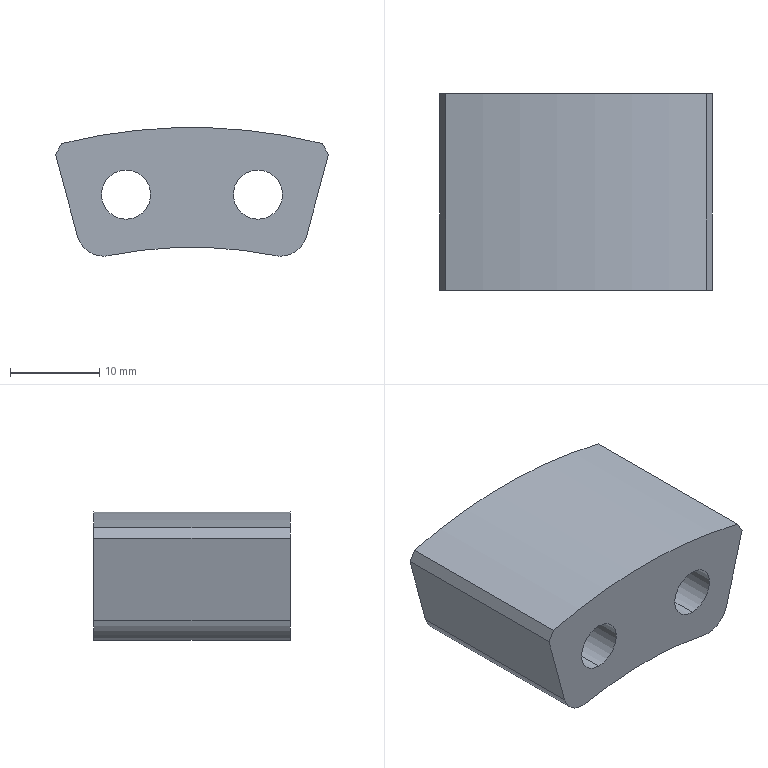Part | SolidWorks | features Chamfer 1, Extrusion 1, Fillet 1, HoleWzd 1, ICE 1 | 1 solid | 22 faces | box 30.541 x 22 x 14.401 mm | volume 6316 mm3 | cylinder 14 | plane 8 | commonest cylinder face diameters 5.5 x4 6 x4 10 x4 93.2 x1 120 x1
STEP:
#1=CARTESIAN_POINT('',(-7.376,15.,47.484));
#2=VERTEX_POINT('',#1);
#3=CARTESIAN_POINT('',(-7.376,15.,57.484));
#4=VERTEX_POINT('',#3);
#5=CARTESIAN_POINT('',(-7.376,15.,52.484));
#6=DIRECTION('',(0.,1.,0.));
#7=DIRECTION('',(0.,0.,1.));
#8=AXIS2_PLACEMENT_3D('',#5,#6,#7);
#9=CIRCLE('',#8,5.);
#10=EDGE_CURVE('',#2,#4,#9,.T.);
#11=ORIENTED_EDGE('',*,*,#10,.F.);
#12=CARTESIAN_POINT('',(-7.376,22.,47.484));
#13=VERTEX_POINT('',#12);
#14=CARTESIAN_POINT('',(-7.376,22.,47.484));
#15=DIRECTION('',(0.,1.,0.));
#16=VECTOR('',#15,1000.);
#17=LINE('',#14,#16);
#18=EDGE_CURVE('',#2,#13,#17,.T.);
#19=ORIENTED_EDGE('',*,*,#18,.T.);
#20=CARTESIAN_POINT('',(-7.376,22.,57.484));
#21=VERTEX_POINT('',#20);
#22=CARTESIAN_POINT('',(-7.376,22.,52.484));
#23=DIRECTION('',(0.,1.,0.));
#24=DIRECTION('',(0.,0.,1.));
#25=AXIS2_PLACEMENT_3D('',#22,#23,#24);
#26=CIRCLE('',#25,5.);
#27=EDGE_CURVE('',#13,#21,#26,.T.);
#28=ORIENTED_EDGE('',*,*,#27,.T.);
#29=CARTESIAN_POINT('',(-7.376,22.,57.484));
#30=DIRECTION('',(0.,1.,0.));
#31=VECTOR('',#30,1000.);
#32=LINE('',#29,#31);
#33=EDGE_CURVE('',#4,#21,#32,.T.);
#34=ORIENTED_EDGE('',*,*,#33,.F.);
#35=EDGE_LOOP('',(#11,#19,#28,#34));
#36=FACE_OUTER_BOUND('',#35,.T.);
#37=CARTESIAN_POINT('',(-7.376,22.,52.484));
#38=DIRECTION('',(0.,1.,0.));
#39=DIRECTION('',(0.,0.,1.));
#40=AXIS2_PLACEMENT_3D('',#37,#38,#39);
#41=CYLINDRICAL_SURFACE('',#40,5.);
#42=ADVANCED_FACE('',(#36),#41,.F.);
#43=CARTESIAN_POINT('',(-7.376,0.,49.734));
#44=VERTEX_POINT('',#43);
#45=CARTESIAN_POINT('',(-7.376,0.,55.234));
#46=VERTEX_POINT('',#45);
#47=CARTESIAN_POINT('',(-7.376,0.,52.484));
#48=DIRECTION('',(0.,1.,0.));
#49=DIRECTION('',(0.,0.,1.));
#50=AXIS2_PLACEMENT_3D('',#47,#48,#49);
#51=CIRCLE('',#50,2.75);
#52=EDGE_CURVE('',#44,#46,#51,.T.);
#53=ORIENTED_EDGE('',*,*,#52,.F.);
#54=CARTESIAN_POINT('',(-7.376,15.,49.734));
#55=VERTEX_POINT('',#54);
#56=CARTESIAN_POINT('',(-7.376,22.,49.734));
#57=DIRECTION('',(0.,1.,0.));
#58=VECTOR('',#57,1000.);
#59=LINE('',#56,#58);
#60=EDGE_CURVE('',#44,#55,#59,.T.);
#61=ORIENTED_EDGE('',*,*,#60,.T.);
#62=CARTESIAN_POINT('',(-7.376,15.,55.234));
#63=VERTEX_POINT('',#62);
#64=CARTESIAN_POINT('',(-7.376,15.,52.484));
#65=DIRECTION('',(0.,1.,0.));
#66=DIRECTION('',(0.,0.,1.));
#67=AXIS2_PLACEMENT_3D('',#64,#65,#66);
#68=CIRCLE('',#67,2.75);
#69=EDGE_CURVE('',#55,#63,#68,.T.);
#70=ORIENTED_EDGE('',*,*,#69,.T.);
#71=CARTESIAN_POINT('',(-7.376,22.,55.234));
#72=DIRECTION('',(0.,1.,0.));
#73=VECTOR('',#72,1000.);
#74=LINE('',#71,#73);
#75=EDGE_CURVE('',#46,#63,#74,.T.);
#76=ORIENTED_EDGE('',*,*,#75,.F.);
#77=EDGE_LOOP('',(#53,#61,#70,#76));
#78=FACE_OUTER_BOUND('',#77,.T.);
#79=CARTESIAN_POINT('',(-7.376,22.,52.484));
#80=DIRECTION('',(0.,1.,0.));
#81=DIRECTION('',(0.,0.,1.));
#82=AXIS2_PLACEMENT_3D('',#79,#80,#81);
#83=CYLINDRICAL_SURFACE('',#82,2.75);
#84=ADVANCED_FACE('',(#78),#83,.F.);
#85=CARTESIAN_POINT('',(7.376,15.,47.484));
#86=VERTEX_POINT('',#85);
#87=CARTESIAN_POINT('',(7.376,15.,57.484));
#88=VERTEX_POINT('',#87);
#89=CARTESIAN_POINT('',(7.376,15.,52.484));
#90=DIRECTION('',(0.,1.,0.));
#91=DIRECTION('',(0.,0.,1.));
#92=AXIS2_PLACEMENT_3D('',#89,#90,#91);
#93=CIRCLE('',#92,5.);
#94=EDGE_CURVE('',#86,#88,#93,.T.);
#95=ORIENTED_EDGE('',*,*,#94,.F.);
#96=CARTESIAN_POINT('',(7.376,22.,47.484));
#97=VERTEX_POINT('',#96);
#98=CARTESIAN_POINT('',(7.376,22.,47.484));
#99=DIRECTION('',(0.,1.,0.));
#100=VECTOR('',#99,1000.);
#101=LINE('',#98,#100);
#102=EDGE_CURVE('',#86,#97,#101,.T.);
#103=ORIENTED_EDGE('',*,*,#102,.T.);
#104=CARTESIAN_POINT('',(7.376,22.,57.484));
#105=VERTEX_POINT('',#104);
#106=CARTESIAN_POINT('',(7.376,22.,52.484));
#107=DIRECTION('',(0.,1.,0.));
#108=DIRECTION('',(0.,0.,1.));
#109=AXIS2_PLACEMENT_3D('',#106,#107,#108);
#110=CIRCLE('',#109,5.);
#111=EDGE_CURVE('',#97,#105,#110,.T.);
#112=ORIENTED_EDGE('',*,*,#111,.T.);
#113=CARTESIAN_POINT('',(7.376,22.,57.484));
#114=DIRECTION('',(0.,1.,0.));
#115=VECTOR('',#114,1000.);
#116=LINE('',#113,#115);
#117=EDGE_CURVE('',#88,#105,#116,.T.);
#118=ORIENTED_EDGE('',*,*,#117,.F.);
#119=EDGE_LOOP('',(#95,#103,#112,#118));
#120=FACE_OUTER_BOUND('',#119,.T.);
#121=CARTESIAN_POINT('',(7.376,22.,52.484));
#122=DIRECTION('',(0.,1.,0.));
#123=DIRECTION('',(0.,0.,1.));
#124=AXIS2_PLACEMENT_3D('',#121,#122,#123);
#125=CYLINDRICAL_SURFACE('',#124,5.);
#126=ADVANCED_FACE('',(#120),#125,.F.);
#127=CARTESIAN_POINT('',(7.376,0.,49.734));
#128=VERTEX_POINT('',#127);
#129=CARTESIAN_POINT('',(7.376,0.,55.234));
#130=VERTEX_POINT('',#129);
#131=CARTESIAN_POINT('',(7.376,0.,52.484));
#132=DIRECTION('',(0.,1.,0.));
#133=DIRECTION('',(0.,0.,1.));
#134=AXIS2_PLACEMENT_3D('',#131,#132,#133);
#135=CIRCLE('',#134,2.75);
#136=EDGE_CURVE('',#128,#130,#135,.T.);
#137=ORIENTED_EDGE('',*,*,#136,.F.);
#138=CARTESIAN_POINT('',(7.376,15.,49.734));
#139=VERTEX_POINT('',#138);
#140=CARTESIAN_POINT('',(7.376,22.,49.734));
#141=DIRECTION('',(0.,1.,0.));
#142=VECTOR('',#141,1000.);
#143=LINE('',#140,#142);
#144=EDGE_CURVE('',#128,#139,#143,.T.);
#145=ORIENTED_EDGE('',*,*,#144,.T.);
#146=CARTESIAN_POINT('',(7.376,15.,55.234));
#147=VERTEX_POINT('',#146);
#148=CARTESIAN_POINT('',(7.376,15.,52.484));
#149=DIRECTION('',(0.,1.,0.));
#150=DIRECTION('',(0.,0.,1.));
#151=AXIS2_PLACEMENT_3D('',#148,#149,#150);
#152=CIRCLE('',#151,2.75);
#153=EDGE_CURVE('',#139,#147,#152,.T.);
#154=ORIENTED_EDGE('',*,*,#153,.T.);
#155=CARTESIAN_POINT('',(7.376,22.,55.234));
#156=DIRECTION('',(0.,1.,0.));
#157=VECTOR('',#156,1000.);
#158=LINE('',#155,#157);
#159=EDGE_CURVE('',#130,#147,#158,.T.);
#160=ORIENTED_EDGE('',*,*,#159,.F.);
#161=EDGE_LOOP('',(#137,#145,#154,#160));
#162=FACE_OUTER_BOUND('',#161,.T.);
#163=CARTESIAN_POINT('',(7.376,22.,52.484));
#164=DIRECTION('',(0.,1.,0.));
#165=DIRECTION('',(0.,0.,1.));
#166=AXIS2_PLACEMENT_3D('',#163,#164,#165);
#167=CYLINDRICAL_SURFACE('',#166,2.75);
#168=ADVANCED_FACE('',(#162),#167,.F.);
#169=CARTESIAN_POINT('',(9.916,22.,45.599));
#170=VERTEX_POINT('',#169);
#171=CARTESIAN_POINT('',(9.316,22.,45.659));
#172=VERTEX_POINT('',#171);
#173=CARTESIAN_POINT('',(9.916,22.,48.599));
#174=DIRECTION('',(0.,1.,0.));
#175=DIRECTION('',(0.,0.,1.));
#176=AXIS2_PLACEMENT_3D('',#173,#174,#175);
#177=CIRCLE('',#176,3.);
#178=EDGE_CURVE('',#170,#172,#177,.T.);
#179=ORIENTED_EDGE('',*,*,#178,.F.);
#180=CARTESIAN_POINT('',(9.916,0.,45.599));
#181=VERTEX_POINT('',#180);
#182=CARTESIAN_POINT('',(9.916,22.,45.599));
#183=DIRECTION('',(0.,-1.,0.));
#184=VECTOR('',#183,1000.);
#185=LINE('',#182,#184);
#186=EDGE_CURVE('',#170,#181,#185,.T.);
#187=ORIENTED_EDGE('',*,*,#186,.T.);
#188=CARTESIAN_POINT('',(9.316,0.,45.659));
#189=VERTEX_POINT('',#188);
#190=CARTESIAN_POINT('',(9.916,0.,48.599));
#191=DIRECTION('',(0.,-1.,0.));
#192=DIRECTION('',(0.,0.,1.));
#193=AXIS2_PLACEMENT_3D('',#190,#191,#192);
#194=CIRCLE('',#193,3.);
#195=EDGE_CURVE('',#189,#181,#194,.T.);
#196=ORIENTED_EDGE('',*,*,#195,.F.);
#197=CARTESIAN_POINT('',(9.316,22.,45.659));
#198=DIRECTION('',(0.,-1.,0.));
#199=VECTOR('',#198,1000.);
#200=LINE('',#197,#199);
#201=EDGE_CURVE('',#172,#189,#200,.T.);
#202=ORIENTED_EDGE('',*,*,#201,.F.);
#203=EDGE_LOOP('',(#179,#187,#196,#202));
#204=FACE_OUTER_BOUND('',#203,.T.);
#205=CARTESIAN_POINT('',(9.916,22.,48.599));
#206=DIRECTION('',(0.,-1.,0.));
#207=DIRECTION('',(0.,0.,-1.));
#208=AXIS2_PLACEMENT_3D('',#205,#206,#207);
#209=CYLINDRICAL_SURFACE('',#208,3.);
#210=ADVANCED_FACE('',(#204),#209,.T.);
#211=CARTESIAN_POINT('',(-9.916,22.,45.599));
#212=VERTEX_POINT('',#211);
#213=CARTESIAN_POINT('',(-12.814,22.,47.822));
#214=VERTEX_POINT('',#213);
#215=CARTESIAN_POINT('',(-9.916,22.,48.599));
#216=DIRECTION('',(0.,1.,0.));
#217=DIRECTION('',(0.,0.,1.));
#218=AXIS2_PLACEMENT_3D('',#215,#216,#217);
#219=CIRCLE('',#218,3.);
#220=EDGE_CURVE('',#212,#214,#219,.T.);
#221=ORIENTED_EDGE('',*,*,#220,.F.);
#222=CARTESIAN_POINT('',(-9.916,0.,45.599));
#223=VERTEX_POINT('',#222);
#224=CARTESIAN_POINT('',(-9.916,22.,45.599));
#225=DIRECTION('',(0.,-1.,0.));
#226=VECTOR('',#225,1000.);
#227=LINE('',#224,#226);
#228=EDGE_CURVE('',#212,#223,#227,.T.);
#229=ORIENTED_EDGE('',*,*,#228,.T.);
#230=CARTESIAN_POINT('',(-12.814,0.,47.822));
#231=VERTEX_POINT('',#230);
#232=CARTESIAN_POINT('',(-9.916,0.,48.599));
#233=DIRECTION('',(0.,-1.,0.));
#234=DIRECTION('',(0.,0.,1.));
#235=AXIS2_PLACEMENT_3D('',#232,#233,#234);
#236=CIRCLE('',#235,3.);
#237=EDGE_CURVE('',#231,#223,#236,.T.);
#238=ORIENTED_EDGE('',*,*,#237,.F.);
#239=CARTESIAN_POINT('',(-12.814,0.,47.822));
#240=DIRECTION('',(0.,-1.,0.));
#241=VECTOR('',#240,1000.);
#242=LINE('',#239,#241);
#243=EDGE_CURVE('',#214,#231,#242,.T.);
#244=ORIENTED_EDGE('',*,*,#243,.F.);
#245=EDGE_LOOP('',(#221,#229,#238,#244));
#246=FACE_OUTER_BOUND('',#245,.T.);
#247=CARTESIAN_POINT('',(-9.916,22.,48.599));
#248=DIRECTION('',(0.,-1.,0.));
#249=DIRECTION('',(0.,0.,-1.));
#250=AXIS2_PLACEMENT_3D('',#247,#248,#249);
#251=CYLINDRICAL_SURFACE('',#250,3.);
#252=ADVANCED_FACE('',(#246),#251,.T.);
#253=CARTESIAN_POINT('',(-7.376,22.,52.484));
#254=DIRECTION('',(0.,1.,0.));
#255=DIRECTION('',(0.,0.,1.));
#256=AXIS2_PLACEMENT_3D('',#253,#254,#255);
#257=CIRCLE('',#256,5.);
#258=EDGE_CURVE('',#21,#13,#257,.T.);
#259=ORIENTED_EDGE('',*,*,#258,.F.);
#260=ORIENTED_EDGE('',*,*,#27,.F.);
#261=EDGE_LOOP('',(#259,#260));
#262=FACE_BOUND('',#261,.T.);
#263=CARTESIAN_POINT('',(7.376,22.,52.484));
#264=DIRECTION('',(0.,1.,0.));
#265=DIRECTION('',(0.,0.,1.));
#266=AXIS2_PLACEMENT_3D('',#263,#264,#265);
#267=CIRCLE('',#266,5.);
#268=EDGE_CURVE('',#105,#97,#267,.T.);
#269=ORIENTED_EDGE('',*,*,#268,.F.);
#270=ORIENTED_EDGE('',*,*,#111,.F.);
#271=EDGE_LOOP('',(#269,#270));
#272=FACE_BOUND('',#271,.T.);
#273=CARTESIAN_POINT('',(-15.27,22.,56.99));
#274=VERTEX_POINT('',#273);
#275=CARTESIAN_POINT('',(-12.061,22.,45.012));
#276=DIRECTION('',(-0.2588,0.,0.9659));
#277=VECTOR('',#276,1000.);
#278=LINE('',#275,#277);
#279=EDGE_CURVE('',#214,#274,#278,.T.);
#280=ORIENTED_EDGE('',*,*,#279,.T.);
#281=CARTESIAN_POINT('',(-14.569,22.,58.204));
#282=VERTEX_POINT('',#281);
#283=CARTESIAN_POINT('',(-36.13,22.,20.86));
#284=DIRECTION('',(0.5,0.,0.866));
#285=VECTOR('',#284,1000.);
#286=LINE('',#283,#285);
#287=EDGE_CURVE('',#274,#282,#286,.T.);
#288=ORIENTED_EDGE('',*,*,#287,.T.);
#289=CARTESIAN_POINT('',(14.569,22.,58.204));
#290=VERTEX_POINT('',#289);
#291=CARTESIAN_POINT('',(0.,22.,0.));
#292=DIRECTION('',(0.,1.,0.));
#293=DIRECTION('',(0.,0.,1.));
#294=AXIS2_PLACEMENT_3D('',#291,#292,#293);
#295=CIRCLE('',#294,60.);
#296=EDGE_CURVE('',#282,#290,#295,.T.);
#297=ORIENTED_EDGE('',*,*,#296,.T.);
#298=CARTESIAN_POINT('',(15.27,22.,56.99));
#299=VERTEX_POINT('',#298);
#300=CARTESIAN_POINT('',(36.13,22.,20.86));
#301=DIRECTION('',(0.5,0.,-0.866));
#302=VECTOR('',#301,1000.);
#303=LINE('',#300,#302);
#304=EDGE_CURVE('',#290,#299,#303,.T.);
#305=ORIENTED_EDGE('',*,*,#304,.T.);
#306=CARTESIAN_POINT('',(12.814,22.,47.822));
#307=VERTEX_POINT('',#306);
#308=CARTESIAN_POINT('',(12.061,22.,45.012));
#309=DIRECTION('',(-0.2588,0.,-0.9659));
#310=VECTOR('',#309,1000.);
#311=LINE('',#308,#310);
#312=EDGE_CURVE('',#299,#307,#311,.T.);
#313=ORIENTED_EDGE('',*,*,#312,.T.);
#314=CARTESIAN_POINT('',(9.916,22.,48.599));
#315=DIRECTION('',(0.,1.,0.));
#316=DIRECTION('',(0.,0.,1.));
#317=AXIS2_PLACEMENT_3D('',#314,#315,#316);
#318=CIRCLE('',#317,3.);
#319=EDGE_CURVE('',#307,#170,#318,.T.);
#320=ORIENTED_EDGE('',*,*,#319,.T.);
#321=ORIENTED_EDGE('',*,*,#178,.T.);
#322=CARTESIAN_POINT('',(-9.316,22.,45.659));
#323=VERTEX_POINT('',#322);
#324=CARTESIAN_POINT('',(0.,22.,0.));
#325=DIRECTION('',(0.,1.,0.));
#326=DIRECTION('',(0.,0.,1.));
#327=AXIS2_PLACEMENT_3D('',#324,#325,#326);
#328=CIRCLE('',#327,46.6);
#329=EDGE_CURVE('',#323,#172,#328,.T.);
#330=ORIENTED_EDGE('',*,*,#329,.F.);
#331=CARTESIAN_POINT('',(-9.916,22.,48.599));
#332=DIRECTION('',(0.,1.,0.));
#333=DIRECTION('',(0.,0.,1.));
#334=AXIS2_PLACEMENT_3D('',#331,#332,#333);
#335=CIRCLE('',#334,3.);
#336=EDGE_CURVE('',#323,#212,#335,.T.);
#337=ORIENTED_EDGE('',*,*,#336,.T.);
#338=ORIENTED_EDGE('',*,*,#220,.T.);
#339=EDGE_LOOP('',(#280,#288,#297,#305,#313,#320,#321,#330,#337,#338));
#340=FACE_OUTER_BOUND('',#339,.T.);
#341=CARTESIAN_POINT('',(0.,22.,0.));
#342=DIRECTION('',(0.,1.,0.));
#343=DIRECTION('',(0.,0.,1.));
#344=AXIS2_PLACEMENT_3D('',#341,#342,#343);
#345=PLANE('',#344);
#346=ADVANCED_FACE('',(#262,#272,#340),#345,.T.);
#347=CARTESIAN_POINT('',(-7.376,0.,52.484));
#348=DIRECTION('',(0.,1.,0.));
#349=DIRECTION('',(0.,0.,1.));
#350=AXIS2_PLACEMENT_3D('',#347,#348,#349);
#351=CIRCLE('',#350,2.75);
#352=EDGE_CURVE('',#46,#44,#351,.T.);
#353=ORIENTED_EDGE('',*,*,#352,.T.);
#354=ORIENTED_EDGE('',*,*,#52,.T.);
#355=EDGE_LOOP('',(#353,#354));
#356=FACE_BOUND('',#355,.T.);
#357=CARTESIAN_POINT('',(7.376,0.,52.484));
#358=DIRECTION('',(0.,1.,0.));
#359=DIRECTION('',(0.,0.,1.));
#360=AXIS2_PLACEMENT_3D('',#357,#358,#359);
#361=CIRCLE('',#360,2.75);
#362=EDGE_CURVE('',#130,#128,#361,.T.);
#363=ORIENTED_EDGE('',*,*,#362,.T.);
#364=ORIENTED_EDGE('',*,*,#136,.T.);
#365=EDGE_LOOP('',(#363,#364));
#366=FACE_BOUND('',#365,.T.);
#367=CARTESIAN_POINT('',(-14.569,0.,58.204));
#368=VERTEX_POINT('',#367);
#369=CARTESIAN_POINT('',(14.569,0.,58.204));
#370=VERTEX_POINT('',#369);
#371=CARTESIAN_POINT('',(0.,0.,0.));
#372=DIRECTION('',(0.,1.,0.));
#373=DIRECTION('',(0.,0.,1.));
#374=AXIS2_PLACEMENT_3D('',#371,#372,#373);
#375=CIRCLE('',#374,60.);
#376=EDGE_CURVE('',#368,#370,#375,.T.);
#377=ORIENTED_EDGE('',*,*,#376,.F.);
#378=CARTESIAN_POINT('',(-15.27,0.,56.99));
#379=VERTEX_POINT('',#378);
#380=CARTESIAN_POINT('',(-15.27,0.,56.99));
#381=DIRECTION('',(-0.5,0.,-0.866));
#382=VECTOR('',#381,1000.);
#383=LINE('',#380,#382);
#384=EDGE_CURVE('',#368,#379,#383,.T.);
#385=ORIENTED_EDGE('',*,*,#384,.T.);
#386=CARTESIAN_POINT('',(-12.061,0.,45.012));
#387=DIRECTION('',(-0.2588,0.,0.9659));
#388=VECTOR('',#387,1000.);
#389=LINE('',#386,#388);
#390=EDGE_CURVE('',#231,#379,#389,.T.);
#391=ORIENTED_EDGE('',*,*,#390,.F.);
#392=ORIENTED_EDGE('',*,*,#237,.T.);
#393=CARTESIAN_POINT('',(-9.316,0.,45.659));
#394=VERTEX_POINT('',#393);
#395=CARTESIAN_POINT('',(-9.916,0.,48.599));
#396=DIRECTION('',(0.,-1.,0.));
#397=DIRECTION('',(0.,0.,1.));
#398=AXIS2_PLACEMENT_3D('',#395,#396,#397);
#399=CIRCLE('',#398,3.);
#400=EDGE_CURVE('',#223,#394,#399,.T.);
#401=ORIENTED_EDGE('',*,*,#400,.T.);
#402=CARTESIAN_POINT('',(0.,0.,0.));
#403=DIRECTION('',(0.,1.,0.));
#404=DIRECTION('',(0.,0.,1.));
#405=AXIS2_PLACEMENT_3D('',#402,#403,#404);
#406=CIRCLE('',#405,46.6);
#407=EDGE_CURVE('',#394,#189,#406,.T.);
#408=ORIENTED_EDGE('',*,*,#407,.T.);
#409=ORIENTED_EDGE('',*,*,#195,.T.);
#410=CARTESIAN_POINT('',(12.814,0.,47.822));
#411=VERTEX_POINT('',#410);
#412=CARTESIAN_POINT('',(9.916,0.,48.599));
#413=DIRECTION('',(0.,-1.,0.));
#414=DIRECTION('',(0.,0.,1.));
#415=AXIS2_PLACEMENT_3D('',#412,#413,#414);
#416=CIRCLE('',#415,3.);
#417=EDGE_CURVE('',#181,#411,#416,.T.);
#418=ORIENTED_EDGE('',*,*,#417,.T.);
#419=CARTESIAN_POINT('',(15.27,0.,56.99));
#420=VERTEX_POINT('',#419);
#421=CARTESIAN_POINT('',(12.061,0.,45.012));
#422=DIRECTION('',(-0.2588,0.,-0.9659));
#423=VECTOR('',#422,1000.);
#424=LINE('',#421,#423);
#425=EDGE_CURVE('',#420,#411,#424,.T.);
#426=ORIENTED_EDGE('',*,*,#425,.F.);
#427=CARTESIAN_POINT('',(14.569,0.,58.204));
#428=DIRECTION('',(-0.5,0.,0.866));
#429=VECTOR('',#428,1000.);
#430=LINE('',#427,#429);
#431=EDGE_CURVE('',#420,#370,#430,.T.);
#432=ORIENTED_EDGE('',*,*,#431,.T.);
#433=EDGE_LOOP('',(#377,#385,#391,#392,#401,#408,#409,#418,#426,#432));
#434=FACE_OUTER_BOUND('',#433,.T.);
#435=CARTESIAN_POINT('',(0.,0.,0.));
#436=DIRECTION('',(0.,1.,0.));
#437=DIRECTION('',(0.,0.,1.));
#438=AXIS2_PLACEMENT_3D('',#435,#436,#437);
#439=PLANE('',#438);
#440=ADVANCED_FACE('',(#356,#366,#434),#439,.F.);
#441=ORIENTED_EDGE('',*,*,#296,.F.);
#442=CARTESIAN_POINT('',(-14.569,22.,58.204));
#443=DIRECTION('',(0.,-1.,0.));
#444=VECTOR('',#443,1000.);
#445=LINE('',#442,#444);
#446=EDGE_CURVE('',#282,#368,#445,.T.);
#447=ORIENTED_EDGE('',*,*,#446,.T.);
#448=ORIENTED_EDGE('',*,*,#376,.T.);
#449=CARTESIAN_POINT('',(14.569,22.,58.204));
#450=DIRECTION('',(0.,1.,0.));
#451=VECTOR('',#450,1000.);
#452=LINE('',#449,#451);
#453=EDGE_CURVE('',#370,#290,#452,.T.);
#454=ORIENTED_EDGE('',*,*,#453,.T.);
#455=EDGE_LOOP('',(#441,#447,#448,#454));
#456=FACE_OUTER_BOUND('',#455,.T.);
#457=CARTESIAN_POINT('',(0.,22.,0.));
#458=DIRECTION('',(0.,-1.,0.));
#459=DIRECTION('',(0.,0.,-1.));
#460=AXIS2_PLACEMENT_3D('',#457,#458,#459);
#461=CYLINDRICAL_SURFACE('',#460,60.);
#462=ADVANCED_FACE('',(#456),#461,.T.);
#463=ORIENTED_EDGE('',*,*,#407,.F.);
#464=CARTESIAN_POINT('',(-9.316,22.,45.659));
#465=DIRECTION('',(0.,1.,0.));
#466=VECTOR('',#465,1000.);
#467=LINE('',#464,#466);
#468=EDGE_CURVE('',#394,#323,#467,.T.);
#469=ORIENTED_EDGE('',*,*,#468,.T.);
#470=ORIENTED_EDGE('',*,*,#329,.T.);
#471=ORIENTED_EDGE('',*,*,#201,.T.);
#472=EDGE_LOOP('',(#463,#469,#470,#471));
#473=FACE_OUTER_BOUND('',#472,.T.);
#474=CARTESIAN_POINT('',(0.,22.,0.));
#475=DIRECTION('',(0.,-1.,0.));
#476=DIRECTION('',(0.,0.,-1.));
#477=AXIS2_PLACEMENT_3D('',#474,#475,#476);
#478=CYLINDRICAL_SURFACE('',#477,46.6);
#479=ADVANCED_FACE('',(#473),#478,.F.);
#480=ORIENTED_EDGE('',*,*,#312,.F.);
#481=CARTESIAN_POINT('',(15.27,0.,56.99));
#482=DIRECTION('',(0.,-1.,0.));
#483=VECTOR('',#482,1000.);
#484=LINE('',#481,#483);
#485=EDGE_CURVE('',#299,#420,#484,.T.);
#486=ORIENTED_EDGE('',*,*,#485,.T.);
#487=ORIENTED_EDGE('',*,*,#425,.T.);
#488=CARTESIAN_POINT('',(12.814,0.,47.822));
#489=DIRECTION('',(0.,1.,0.));
#490=VECTOR('',#489,1000.);
#491=LINE('',#488,#490);
#492=EDGE_CURVE('',#411,#307,#491,.T.);
#493=ORIENTED_EDGE('',*,*,#492,.T.);
#494=EDGE_LOOP('',(#480,#486,#487,#493));
#495=FACE_OUTER_BOUND('',#494,.T.);
#496=CARTESIAN_POINT('',(12.061,0.,45.012));
#497=DIRECTION('',(0.9659,0.,-0.2588));
#498=DIRECTION('',(-0.2588,0.,-0.9659));
#499=AXIS2_PLACEMENT_3D('',#496,#497,#498);
#500=PLANE('',#499);
#501=ADVANCED_FACE('',(#495),#500,.T.);
#502=ORIENTED_EDGE('',*,*,#390,.T.);
#503=CARTESIAN_POINT('',(-15.27,22.,56.99));
#504=DIRECTION('',(0.,1.,0.));
#505=VECTOR('',#504,1000.);
#506=LINE('',#503,#505);
#507=EDGE_CURVE('',#379,#274,#506,.T.);
#508=ORIENTED_EDGE('',*,*,#507,.T.);
#509=ORIENTED_EDGE('',*,*,#279,.F.);
#510=ORIENTED_EDGE('',*,*,#243,.T.);
#511=EDGE_LOOP('',(#502,#508,#509,#510));
#512=FACE_OUTER_BOUND('',#511,.T.);
#513=CARTESIAN_POINT('',(-12.061,0.,45.012));
#514=DIRECTION('',(-0.9659,0.,-0.2588));
#515=DIRECTION('',(-0.2588,0.,0.9659));
#516=AXIS2_PLACEMENT_3D('',#513,#514,#515);
#517=PLANE('',#516);
#518=ADVANCED_FACE('',(#512),#517,.T.);
#519=ORIENTED_EDGE('',*,*,#228,.F.);
#520=ORIENTED_EDGE('',*,*,#336,.F.);
#521=ORIENTED_EDGE('',*,*,#468,.F.);
#522=ORIENTED_EDGE('',*,*,#400,.F.);
#523=EDGE_LOOP('',(#519,#520,#521,#522));
#524=FACE_OUTER_BOUND('',#523,.T.);
#525=CARTESIAN_POINT('',(-9.916,22.,48.599));
#526=DIRECTION('',(0.,-1.,0.));
#527=DIRECTION('',(0.,0.,-1.));
#528=AXIS2_PLACEMENT_3D('',#525,#526,#527);
#529=CYLINDRICAL_SURFACE('',#528,3.);
#530=ADVANCED_FACE('',(#524),#529,.T.);
#531=ORIENTED_EDGE('',*,*,#186,.F.);
#532=ORIENTED_EDGE('',*,*,#319,.F.);
#533=ORIENTED_EDGE('',*,*,#492,.F.);
#534=ORIENTED_EDGE('',*,*,#417,.F.);
#535=EDGE_LOOP('',(#531,#532,#533,#534));
#536=FACE_OUTER_BOUND('',#535,.T.);
#537=CARTESIAN_POINT('',(9.916,22.,48.599));
#538=DIRECTION('',(0.,-1.,0.));
#539=DIRECTION('',(0.,0.,-1.));
#540=AXIS2_PLACEMENT_3D('',#537,#538,#539);
#541=CYLINDRICAL_SURFACE('',#540,3.);
#542=ADVANCED_FACE('',(#536),#541,.T.);
#543=ORIENTED_EDGE('',*,*,#384,.F.);
#544=ORIENTED_EDGE('',*,*,#446,.F.);
#545=ORIENTED_EDGE('',*,*,#287,.F.);
#546=ORIENTED_EDGE('',*,*,#507,.F.);
#547=EDGE_LOOP('',(#543,#544,#545,#546));
#548=FACE_OUTER_BOUND('',#547,.T.);
#549=CARTESIAN_POINT('',(-15.27,22.,56.99));
#550=DIRECTION('',(-0.866,0.,0.5));
#551=DIRECTION('',(0.,-1.,0.));
#552=AXIS2_PLACEMENT_3D('',#549,#550,#551);
#553=PLANE('',#552);
#554=ADVANCED_FACE('',(#548),#553,.T.);
#555=ORIENTED_EDGE('',*,*,#431,.F.);
#556=ORIENTED_EDGE('',*,*,#485,.F.);
#557=ORIENTED_EDGE('',*,*,#304,.F.);
#558=ORIENTED_EDGE('',*,*,#453,.F.);
#559=EDGE_LOOP('',(#555,#556,#557,#558));
#560=FACE_OUTER_BOUND('',#559,.T.);
#561=CARTESIAN_POINT('',(14.569,22.,58.204));
#562=DIRECTION('',(0.866,0.,0.5));
#563=DIRECTION('',(0.,-1.,0.));
#564=AXIS2_PLACEMENT_3D('',#561,#562,#563);
#565=PLANE('',#564);
#566=ADVANCED_FACE('',(#560),#565,.T.);
#567=ORIENTED_EDGE('',*,*,#144,.F.);
#568=ORIENTED_EDGE('',*,*,#362,.F.);
#569=ORIENTED_EDGE('',*,*,#159,.T.);
#570=CARTESIAN_POINT('',(7.376,15.,52.484));
#571=DIRECTION('',(0.,1.,0.));
#572=DIRECTION('',(0.,0.,1.));
#573=AXIS2_PLACEMENT_3D('',#570,#571,#572);
#574=CIRCLE('',#573,2.75);
#575=EDGE_CURVE('',#147,#139,#574,.T.);
#576=ORIENTED_EDGE('',*,*,#575,.T.);
#577=EDGE_LOOP('',(#567,#568,#569,#576));
#578=FACE_OUTER_BOUND('',#577,.T.);
#579=CARTESIAN_POINT('',(7.376,22.,52.484));
#580=DIRECTION('',(0.,1.,0.));
#581=DIRECTION('',(0.,0.,1.));
#582=AXIS2_PLACEMENT_3D('',#579,#580,#581);
#583=CYLINDRICAL_SURFACE('',#582,2.75);
#584=ADVANCED_FACE('',(#578),#583,.F.);
#585=ORIENTED_EDGE('',*,*,#575,.F.);
#586=ORIENTED_EDGE('',*,*,#153,.F.);
#587=EDGE_LOOP('',(#585,#586));
#588=FACE_BOUND('',#587,.T.);
#589=CARTESIAN_POINT('',(7.376,15.,52.484));
#590=DIRECTION('',(0.,1.,0.));
#591=DIRECTION('',(0.,0.,1.));
#592=AXIS2_PLACEMENT_3D('',#589,#590,#591);
#593=CIRCLE('',#592,5.);
#594=EDGE_CURVE('',#88,#86,#593,.T.);
#595=ORIENTED_EDGE('',*,*,#594,.T.);
#596=ORIENTED_EDGE('',*,*,#94,.T.);
#597=EDGE_LOOP('',(#595,#596));
#598=FACE_OUTER_BOUND('',#597,.T.);
#599=CARTESIAN_POINT('',(10.126,15.,52.484));
#600=DIRECTION('',(0.,-1.,0.));
#601=DIRECTION('',(0.,0.,-1.));
#602=AXIS2_PLACEMENT_3D('',#599,#600,#601);
#603=PLANE('',#602);
#604=ADVANCED_FACE('',(#588,#598),#603,.F.);
#605=ORIENTED_EDGE('',*,*,#102,.F.);
#606=ORIENTED_EDGE('',*,*,#594,.F.);
#607=ORIENTED_EDGE('',*,*,#117,.T.);
#608=ORIENTED_EDGE('',*,*,#268,.T.);
#609=EDGE_LOOP('',(#605,#606,#607,#608));
#610=FACE_OUTER_BOUND('',#609,.T.);
#611=CARTESIAN_POINT('',(7.376,22.,52.484));
#612=DIRECTION('',(0.,1.,0.));
#613=DIRECTION('',(0.,0.,1.));
#614=AXIS2_PLACEMENT_3D('',#611,#612,#613);
#615=CYLINDRICAL_SURFACE('',#614,5.);
#616=ADVANCED_FACE('',(#610),#615,.F.);
#617=ORIENTED_EDGE('',*,*,#60,.F.);
#618=ORIENTED_EDGE('',*,*,#352,.F.);
#619=ORIENTED_EDGE('',*,*,#75,.T.);
#620=CARTESIAN_POINT('',(-7.376,15.,52.484));
#621=DIRECTION('',(0.,1.,0.));
#622=DIRECTION('',(0.,0.,1.));
#623=AXIS2_PLACEMENT_3D('',#620,#621,#622);
#624=CIRCLE('',#623,2.75);
#625=EDGE_CURVE('',#63,#55,#624,.T.);
#626=ORIENTED_EDGE('',*,*,#625,.T.);
#627=EDGE_LOOP('',(#617,#618,#619,#626));
#628=FACE_OUTER_BOUND('',#627,.T.);
#629=CARTESIAN_POINT('',(-7.376,22.,52.484));
#630=DIRECTION('',(0.,1.,0.));
#631=DIRECTION('',(0.,0.,1.));
#632=AXIS2_PLACEMENT_3D('',#629,#630,#631);
#633=CYLINDRICAL_SURFACE('',#632,2.75);
#634=ADVANCED_FACE('',(#628),#633,.F.);
#635=ORIENTED_EDGE('',*,*,#625,.F.);
#636=ORIENTED_EDGE('',*,*,#69,.F.);
#637=EDGE_LOOP('',(#635,#636));
#638=FACE_BOUND('',#637,.T.);
#639=CARTESIAN_POINT('',(-7.376,15.,52.484));
#640=DIRECTION('',(0.,1.,0.));
#641=DIRECTION('',(0.,0.,1.));
#642=AXIS2_PLACEMENT_3D('',#639,#640,#641);
#643=CIRCLE('',#642,5.);
#644=EDGE_CURVE('',#4,#2,#643,.T.);
#645=ORIENTED_EDGE('',*,*,#644,.T.);
#646=ORIENTED_EDGE('',*,*,#10,.T.);
#647=EDGE_LOOP('',(#645,#646));
#648=FACE_OUTER_BOUND('',#647,.T.);
#649=CARTESIAN_POINT('',(-4.626,15.,52.484));
#650=DIRECTION('',(0.,-1.,0.));
#651=DIRECTION('',(0.,0.,-1.));
#652=AXIS2_PLACEMENT_3D('',#649,#650,#651);
#653=PLANE('',#652);
#654=ADVANCED_FACE('',(#638,#648),#653,.F.);
#655=ORIENTED_EDGE('',*,*,#18,.F.);
#656=ORIENTED_EDGE('',*,*,#644,.F.);
#657=ORIENTED_EDGE('',*,*,#33,.T.);
#658=ORIENTED_EDGE('',*,*,#258,.T.);
#659=EDGE_LOOP('',(#655,#656,#657,#658));
#660=FACE_OUTER_BOUND('',#659,.T.);
#661=CARTESIAN_POINT('',(-7.376,22.,52.484));
#662=DIRECTION('',(0.,1.,0.));
#663=DIRECTION('',(0.,0.,1.));
#664=AXIS2_PLACEMENT_3D('',#661,#662,#663);
#665=CYLINDRICAL_SURFACE('',#664,5.);
#666=ADVANCED_FACE('',(#660),#665,.F.);
#667=CLOSED_SHELL('',(#42,#84,#126,#168,#210,#252,#346,#440,#462,#479,#501,#518,#530,#542,#554,#566,#584,#604,#616,#634,#654,#666));
#668=MANIFOLD_SOLID_BREP('',#667);
#669=CARTESIAN_POINT('',(0.,0.,0.));
#670=DIRECTION('',(0.,0.,1.));
#671=DIRECTION('',(1.,0.,0.));
#672=AXIS2_PLACEMENT_3D('',#669,#670,#671);
#673=(LENGTH_UNIT()NAMED_UNIT(*)SI_UNIT(.MILLI.,.METRE.));
#674=UNCERTAINTY_MEASURE_WITH_UNIT(LENGTH_MEASURE(0.00001),#673,'','');
#675=(NAMED_UNIT(*)PLANE_ANGLE_UNIT()SI_UNIT($,.RADIAN.));
#676=(NAMED_UNIT(*)SI_UNIT($,.STERADIAN.)SOLID_ANGLE_UNIT());
#677=(GEOMETRIC_REPRESENTATION_CONTEXT(3)GLOBAL_UNCERTAINTY_ASSIGNED_CONTEXT((#674))GLOBAL_UNIT_ASSIGNED_CONTEXT((#673,#675,#676))REPRESENTATION_CONTEXT('',''));
#678=ADVANCED_BREP_SHAPE_REPRESENTATION('',(#668,#672),#677);